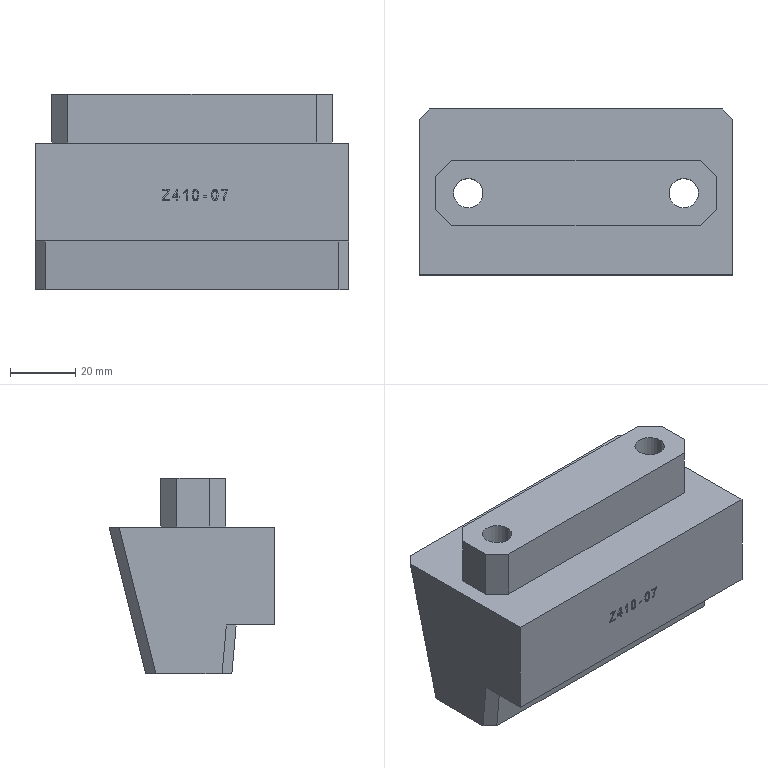Part | Creo | 1 solid | 131 faces | box 96 x 50.783 x 60 mm | volume 192355 mm3 | plane 67 | other 53 | cylinder 11 | commonest cylinder face diameters 9 x4 14 x4 11.472 x1 11.957 x1 45.582 x1